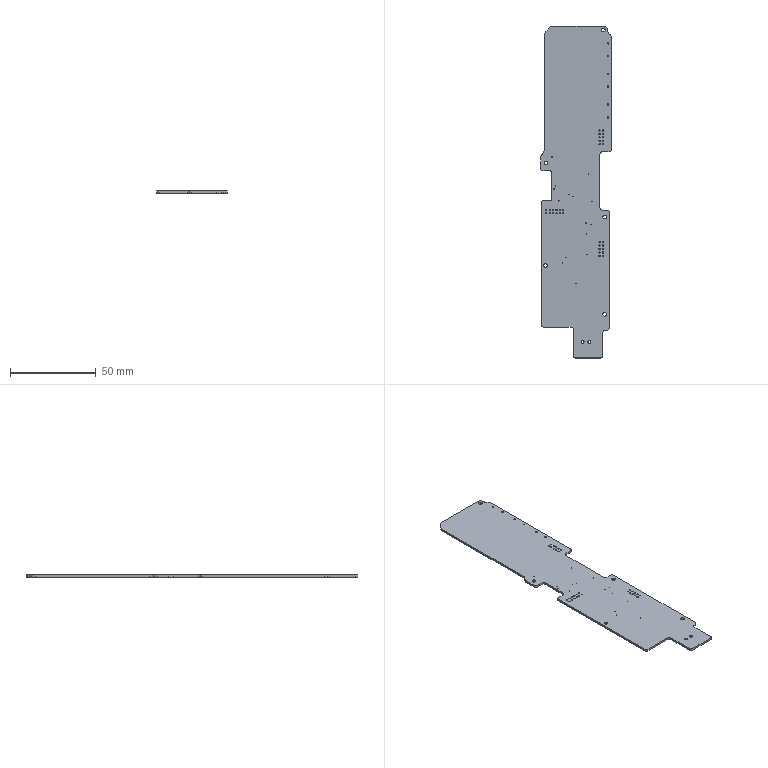Part | STEP file | SOLID | 1 solid | 104 faces | box 40.98 x 193.1 x 1.2 mm | volume 8227 mm3 | cylinder 82 | plane 22 | commonest cylinder face diameters 0.7 x32 0.3 x15 2.54 x14 1 x6 2.1 x5 6.132 x5